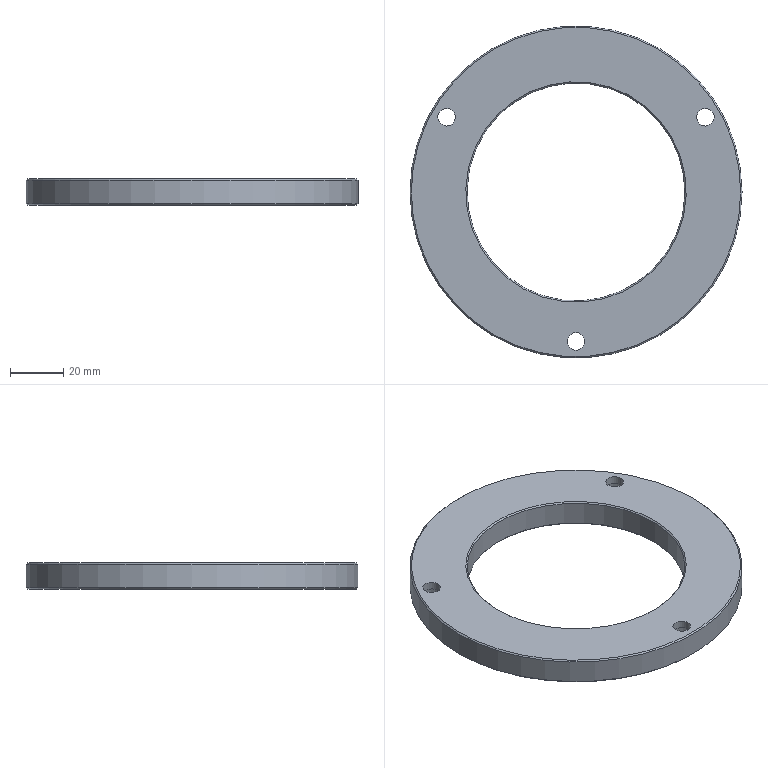Part | STEP file | solid 210 | 1 solid | 17 faces | box 125 x 125 x 10 mm | volume 67442 mm3 | cylinder 8 | plane 5 | cone 4 | commonest cylinder face diameters 6.6 x3 11 x3 82 x1 125 x1